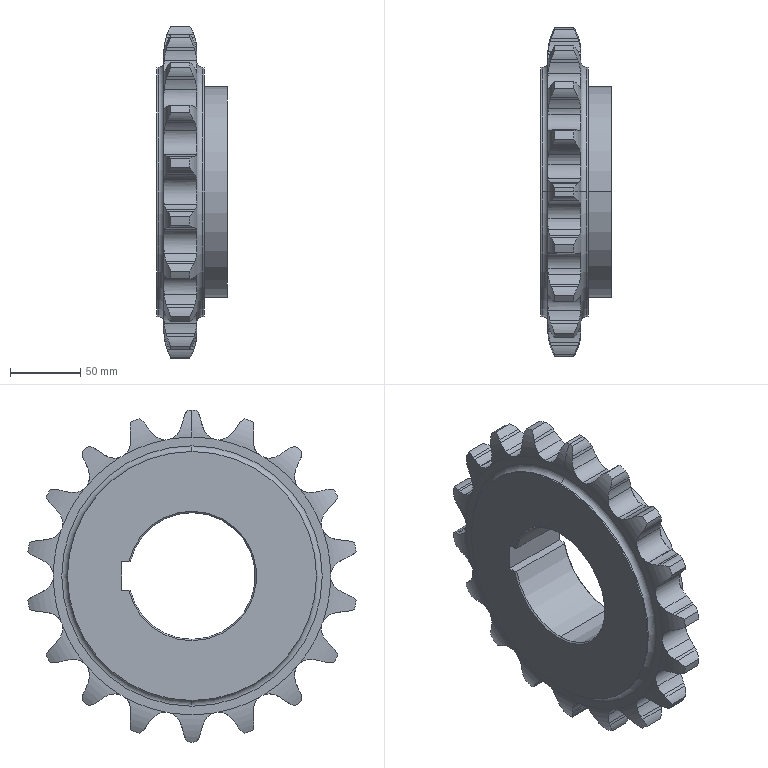Part | SolidWorks | features BaseBody 1 | 1 solid | 218 faces | box 50 x 233.402 x 236 mm | volume 1046718 mm3 | cylinder 126 | plane 44 | torus 42 | cone 6 | commonest cylinder face diameters 32.579 x38 58.009 x36 22.441 x24 236 x19 177 x4 90 x3